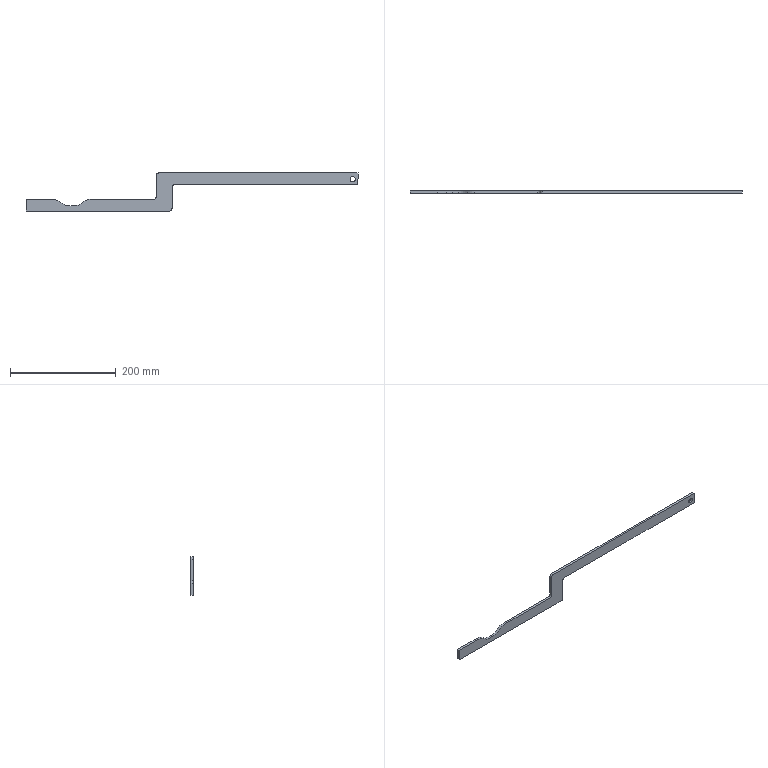Part | SolidWorks | features Extrusion 1 | 1 solid | 24 faces | box 628.5 x 4.5 x 72 mm | volume 66431 mm3 | plane 14 | cylinder 10 | commonest cylinder face diameters 10 x6 40 x4
STEP:
#1=CARTESIAN_POINT('',(618.5,4.5,55.));
#2=VERTEX_POINT('',#1);
#3=CARTESIAN_POINT('',(618.5,4.5,65.));
#4=VERTEX_POINT('',#3);
#5=CARTESIAN_POINT('',(618.5,4.5,60.));
#6=DIRECTION('',(0.,1.,0.));
#7=DIRECTION('',(0.,0.,1.));
#8=AXIS2_PLACEMENT_3D('',#5,#6,#7);
#9=CIRCLE('',#8,5.);
#10=EDGE_CURVE('',#2,#4,#9,.T.);
#11=ORIENTED_EDGE('',*,*,#10,.T.);
#12=CARTESIAN_POINT('',(618.5,0.,65.));
#13=VERTEX_POINT('',#12);
#14=CARTESIAN_POINT('',(618.5,4.5,65.));
#15=DIRECTION('',(0.,-1.,0.));
#16=VECTOR('',#15,1000.);
#17=LINE('',#14,#16);
#18=EDGE_CURVE('',#4,#13,#17,.T.);
#19=ORIENTED_EDGE('',*,*,#18,.T.);
#20=CARTESIAN_POINT('',(618.5,0.,55.));
#21=VERTEX_POINT('',#20);
#22=CARTESIAN_POINT('',(618.5,0.,60.));
#23=DIRECTION('',(0.,1.,0.));
#24=DIRECTION('',(0.,0.,1.));
#25=AXIS2_PLACEMENT_3D('',#22,#23,#24);
#26=CIRCLE('',#25,5.);
#27=EDGE_CURVE('',#21,#13,#26,.T.);
#28=ORIENTED_EDGE('',*,*,#27,.F.);
#29=CARTESIAN_POINT('',(618.5,4.5,55.));
#30=DIRECTION('',(0.,-1.,0.));
#31=VECTOR('',#30,1000.);
#32=LINE('',#29,#31);
#33=EDGE_CURVE('',#2,#21,#32,.T.);
#34=ORIENTED_EDGE('',*,*,#33,.F.);
#35=EDGE_LOOP('',(#11,#19,#28,#34));
#36=FACE_OUTER_BOUND('',#35,.T.);
#37=CARTESIAN_POINT('',(618.5,4.5,60.));
#38=DIRECTION('',(0.,-1.,0.));
#39=DIRECTION('',(0.,0.,-1.));
#40=AXIS2_PLACEMENT_3D('',#37,#38,#39);
#41=CYLINDRICAL_SURFACE('',#40,5.);
#42=ADVANCED_FACE('',(#36),#41,.F.);
#43=CARTESIAN_POINT('',(0.,4.5,0.));
#44=VERTEX_POINT('',#43);
#45=CARTESIAN_POINT('',(0.,4.5,22.));
#46=VERTEX_POINT('',#45);
#47=CARTESIAN_POINT('',(0.,4.5,22.));
#48=DIRECTION('',(0.,0.,1.));
#49=VECTOR('',#48,1000.);
#50=LINE('',#47,#49);
#51=EDGE_CURVE('',#44,#46,#50,.T.);
#52=ORIENTED_EDGE('',*,*,#51,.T.);
#53=CARTESIAN_POINT('',(51.663,4.5,22.));
#54=VERTEX_POINT('',#53);
#55=CARTESIAN_POINT('',(51.663,4.5,22.));
#56=DIRECTION('',(1.,0.,0.));
#57=VECTOR('',#56,1000.);
#58=LINE('',#55,#57);
#59=EDGE_CURVE('',#46,#54,#58,.T.);
#60=ORIENTED_EDGE('',*,*,#59,.T.);
#61=CARTESIAN_POINT('',(63.906,4.5,17.814));
#62=VERTEX_POINT('',#61);
#63=CARTESIAN_POINT('',(51.663,4.5,2.));
#64=DIRECTION('',(0.,1.,0.));
#65=DIRECTION('',(0.,0.,-1.));
#66=AXIS2_PLACEMENT_3D('',#63,#64,#65);
#67=CIRCLE('',#66,20.);
#68=EDGE_CURVE('',#54,#62,#67,.T.);
#69=ORIENTED_EDGE('',*,*,#68,.T.);
#70=CARTESIAN_POINT('',(68.594,4.5,14.186));
#71=VERTEX_POINT('',#70);
#72=CARTESIAN_POINT('',(68.594,4.5,14.186));
#73=DIRECTION('',(0.7907,0.,-0.6122));
#74=VECTOR('',#73,1000.);
#75=LINE('',#72,#74);
#76=EDGE_CURVE('',#62,#71,#75,.T.);
#77=ORIENTED_EDGE('',*,*,#76,.T.);
#78=CARTESIAN_POINT('',(80.837,4.5,10.));
#79=VERTEX_POINT('',#78);
#80=CARTESIAN_POINT('',(80.837,4.5,30.));
#81=DIRECTION('',(0.,-1.,0.));
#82=DIRECTION('',(0.,0.,-1.));
#83=AXIS2_PLACEMENT_3D('',#80,#81,#82);
#84=CIRCLE('',#83,20.);
#85=EDGE_CURVE('',#71,#79,#84,.T.);
#86=ORIENTED_EDGE('',*,*,#85,.T.);
#87=CARTESIAN_POINT('',(92.163,4.5,10.));
#88=VERTEX_POINT('',#87);
#89=CARTESIAN_POINT('',(80.837,4.5,10.));
#90=DIRECTION('',(1.,0.,0.));
#91=VECTOR('',#90,1000.);
#92=LINE('',#89,#91);
#93=EDGE_CURVE('',#79,#88,#92,.T.);
#94=ORIENTED_EDGE('',*,*,#93,.T.);
#95=CARTESIAN_POINT('',(104.406,4.5,14.186));
#96=VERTEX_POINT('',#95);
#97=CARTESIAN_POINT('',(92.163,4.5,30.));
#98=DIRECTION('',(0.,-1.,0.));
#99=DIRECTION('',(0.,0.,-1.));
#100=AXIS2_PLACEMENT_3D('',#97,#98,#99);
#101=CIRCLE('',#100,20.);
#102=EDGE_CURVE('',#88,#96,#101,.T.);
#103=ORIENTED_EDGE('',*,*,#102,.T.);
#104=CARTESIAN_POINT('',(109.094,4.5,17.814));
#105=VERTEX_POINT('',#104);
#106=CARTESIAN_POINT('',(104.406,4.5,14.186));
#107=DIRECTION('',(0.7907,0.,0.6122));
#108=VECTOR('',#107,1000.);
#109=LINE('',#106,#108);
#110=EDGE_CURVE('',#96,#105,#109,.T.);
#111=ORIENTED_EDGE('',*,*,#110,.T.);
#112=CARTESIAN_POINT('',(121.337,4.5,22.));
#113=VERTEX_POINT('',#112);
#114=CARTESIAN_POINT('',(121.337,4.5,2.));
#115=DIRECTION('',(0.,1.,0.));
#116=DIRECTION('',(0.,0.,-1.));
#117=AXIS2_PLACEMENT_3D('',#114,#115,#116);
#118=CIRCLE('',#117,20.);
#119=EDGE_CURVE('',#105,#113,#118,.T.);
#120=ORIENTED_EDGE('',*,*,#119,.T.);
#121=CARTESIAN_POINT('',(241.5,4.5,22.));
#122=VERTEX_POINT('',#121);
#123=CARTESIAN_POINT('',(241.5,4.5,22.));
#124=DIRECTION('',(1.,0.,0.));
#125=VECTOR('',#124,1000.);
#126=LINE('',#123,#125);
#127=EDGE_CURVE('',#113,#122,#126,.T.);
#128=ORIENTED_EDGE('',*,*,#127,.T.);
#129=CARTESIAN_POINT('',(246.5,4.5,27.));
#130=VERTEX_POINT('',#129);
#131=CARTESIAN_POINT('',(241.5,4.5,27.));
#132=DIRECTION('',(0.,-1.,0.));
#133=DIRECTION('',(0.,0.,1.));
#134=AXIS2_PLACEMENT_3D('',#131,#132,#133);
#135=CIRCLE('',#134,5.);
#136=EDGE_CURVE('',#122,#130,#135,.T.);
#137=ORIENTED_EDGE('',*,*,#136,.T.);
#138=CARTESIAN_POINT('',(246.5,4.5,67.));
#139=VERTEX_POINT('',#138);
#140=CARTESIAN_POINT('',(246.5,4.5,67.));
#141=DIRECTION('',(0.,0.,1.));
#142=VECTOR('',#141,1000.);
#143=LINE('',#140,#142);
#144=EDGE_CURVE('',#130,#139,#143,.T.);
#145=ORIENTED_EDGE('',*,*,#144,.T.);
#146=CARTESIAN_POINT('',(251.5,4.5,72.));
#147=VERTEX_POINT('',#146);
#148=CARTESIAN_POINT('',(251.5,4.5,67.));
#149=DIRECTION('',(0.,1.,0.));
#150=DIRECTION('',(0.,0.,-1.));
#151=AXIS2_PLACEMENT_3D('',#148,#149,#150);
#152=CIRCLE('',#151,5.);
#153=EDGE_CURVE('',#139,#147,#152,.T.);
#154=ORIENTED_EDGE('',*,*,#153,.T.);
#155=CARTESIAN_POINT('',(628.5,4.5,72.));
#156=VERTEX_POINT('',#155);
#157=CARTESIAN_POINT('',(628.5,4.5,72.));
#158=DIRECTION('',(1.,0.,0.));
#159=VECTOR('',#158,1000.);
#160=LINE('',#157,#159);
#161=EDGE_CURVE('',#147,#156,#160,.T.);
#162=ORIENTED_EDGE('',*,*,#161,.T.);
#163=CARTESIAN_POINT('',(628.5,4.5,50.));
#164=VERTEX_POINT('',#163);
#165=CARTESIAN_POINT('',(628.5,4.5,50.));
#166=DIRECTION('',(0.,0.,-1.));
#167=VECTOR('',#166,1000.);
#168=LINE('',#165,#167);
#169=EDGE_CURVE('',#156,#164,#168,.T.);
#170=ORIENTED_EDGE('',*,*,#169,.T.);
#171=CARTESIAN_POINT('',(281.5,4.5,50.));
#172=VERTEX_POINT('',#171);
#173=CARTESIAN_POINT('',(281.5,4.5,50.));
#174=DIRECTION('',(-1.,0.,0.));
#175=VECTOR('',#174,1000.);
#176=LINE('',#173,#175);
#177=EDGE_CURVE('',#164,#172,#176,.T.);
#178=ORIENTED_EDGE('',*,*,#177,.T.);
#179=CARTESIAN_POINT('',(276.5,4.5,45.));
#180=VERTEX_POINT('',#179);
#181=CARTESIAN_POINT('',(281.5,4.5,45.));
#182=DIRECTION('',(0.,-1.,0.));
#183=DIRECTION('',(0.,0.,1.));
#184=AXIS2_PLACEMENT_3D('',#181,#182,#183);
#185=CIRCLE('',#184,5.);
#186=EDGE_CURVE('',#172,#180,#185,.T.);
#187=ORIENTED_EDGE('',*,*,#186,.T.);
#188=CARTESIAN_POINT('',(276.5,4.5,5.));
#189=VERTEX_POINT('',#188);
#190=CARTESIAN_POINT('',(276.5,4.5,5.));
#191=DIRECTION('',(0.,0.,-1.));
#192=VECTOR('',#191,1000.);
#193=LINE('',#190,#192);
#194=EDGE_CURVE('',#180,#189,#193,.T.);
#195=ORIENTED_EDGE('',*,*,#194,.T.);
#196=CARTESIAN_POINT('',(271.5,4.5,0.));
#197=VERTEX_POINT('',#196);
#198=CARTESIAN_POINT('',(271.5,4.5,5.));
#199=DIRECTION('',(0.,1.,0.));
#200=DIRECTION('',(0.,0.,-1.));
#201=AXIS2_PLACEMENT_3D('',#198,#199,#200);
#202=CIRCLE('',#201,5.);
#203=EDGE_CURVE('',#189,#197,#202,.T.);
#204=ORIENTED_EDGE('',*,*,#203,.T.);
#205=CARTESIAN_POINT('',(0.,4.5,0.));
#206=DIRECTION('',(-1.,0.,0.));
#207=VECTOR('',#206,1000.);
#208=LINE('',#205,#207);
#209=EDGE_CURVE('',#197,#44,#208,.T.);
#210=ORIENTED_EDGE('',*,*,#209,.T.);
#211=EDGE_LOOP('',(#52,#60,#69,#77,#86,#94,#103,#111,#120,#128,#137,#145,#154,#162,#170,#178,#187,#195,#204,#210));
#212=FACE_OUTER_BOUND('',#211,.T.);
#213=ORIENTED_EDGE('',*,*,#10,.F.);
#214=CARTESIAN_POINT('',(618.5,4.5,60.));
#215=DIRECTION('',(0.,1.,0.));
#216=DIRECTION('',(0.,0.,1.));
#217=AXIS2_PLACEMENT_3D('',#214,#215,#216);
#218=CIRCLE('',#217,5.);
#219=EDGE_CURVE('',#4,#2,#218,.T.);
#220=ORIENTED_EDGE('',*,*,#219,.F.);
#221=EDGE_LOOP('',(#213,#220));
#222=FACE_BOUND('',#221,.T.);
#223=CARTESIAN_POINT('',(271.5,4.5,5.));
#224=DIRECTION('',(0.,-1.,0.));
#225=DIRECTION('',(0.,0.,-1.));
#226=AXIS2_PLACEMENT_3D('',#223,#224,#225);
#227=PLANE('',#226);
#228=ADVANCED_FACE('',(#212,#222),#227,.F.);
#229=CARTESIAN_POINT('',(0.,0.,0.));
#230=VERTEX_POINT('',#229);
#231=CARTESIAN_POINT('',(0.,0.,22.));
#232=VERTEX_POINT('',#231);
#233=CARTESIAN_POINT('',(0.,0.,22.));
#234=DIRECTION('',(0.,0.,1.));
#235=VECTOR('',#234,1000.);
#236=LINE('',#233,#235);
#237=EDGE_CURVE('',#230,#232,#236,.T.);
#238=ORIENTED_EDGE('',*,*,#237,.F.);
#239=CARTESIAN_POINT('',(271.5,0.,0.));
#240=VERTEX_POINT('',#239);
#241=CARTESIAN_POINT('',(0.,0.,0.));
#242=DIRECTION('',(-1.,0.,0.));
#243=VECTOR('',#242,1000.);
#244=LINE('',#241,#243);
#245=EDGE_CURVE('',#240,#230,#244,.T.);
#246=ORIENTED_EDGE('',*,*,#245,.F.);
#247=CARTESIAN_POINT('',(276.5,0.,5.));
#248=VERTEX_POINT('',#247);
#249=CARTESIAN_POINT('',(271.5,0.,5.));
#250=DIRECTION('',(0.,1.,0.));
#251=DIRECTION('',(0.,0.,-1.));
#252=AXIS2_PLACEMENT_3D('',#249,#250,#251);
#253=CIRCLE('',#252,5.);
#254=EDGE_CURVE('',#248,#240,#253,.T.);
#255=ORIENTED_EDGE('',*,*,#254,.F.);
#256=CARTESIAN_POINT('',(276.5,0.,45.));
#257=VERTEX_POINT('',#256);
#258=CARTESIAN_POINT('',(276.5,0.,5.));
#259=DIRECTION('',(0.,0.,-1.));
#260=VECTOR('',#259,1000.);
#261=LINE('',#258,#260);
#262=EDGE_CURVE('',#257,#248,#261,.T.);
#263=ORIENTED_EDGE('',*,*,#262,.F.);
#264=CARTESIAN_POINT('',(281.5,0.,50.));
#265=VERTEX_POINT('',#264);
#266=CARTESIAN_POINT('',(281.5,0.,45.));
#267=DIRECTION('',(0.,-1.,0.));
#268=DIRECTION('',(0.,0.,1.));
#269=AXIS2_PLACEMENT_3D('',#266,#267,#268);
#270=CIRCLE('',#269,5.);
#271=EDGE_CURVE('',#265,#257,#270,.T.);
#272=ORIENTED_EDGE('',*,*,#271,.F.);
#273=CARTESIAN_POINT('',(628.5,0.,50.));
#274=VERTEX_POINT('',#273);
#275=CARTESIAN_POINT('',(281.5,0.,50.));
#276=DIRECTION('',(-1.,0.,0.));
#277=VECTOR('',#276,1000.);
#278=LINE('',#275,#277);
#279=EDGE_CURVE('',#274,#265,#278,.T.);
#280=ORIENTED_EDGE('',*,*,#279,.F.);
#281=CARTESIAN_POINT('',(628.5,0.,72.));
#282=VERTEX_POINT('',#281);
#283=CARTESIAN_POINT('',(628.5,0.,50.));
#284=DIRECTION('',(0.,0.,-1.));
#285=VECTOR('',#284,1000.);
#286=LINE('',#283,#285);
#287=EDGE_CURVE('',#282,#274,#286,.T.);
#288=ORIENTED_EDGE('',*,*,#287,.F.);
#289=CARTESIAN_POINT('',(251.5,0.,72.));
#290=VERTEX_POINT('',#289);
#291=CARTESIAN_POINT('',(628.5,0.,72.));
#292=DIRECTION('',(1.,0.,0.));
#293=VECTOR('',#292,1000.);
#294=LINE('',#291,#293);
#295=EDGE_CURVE('',#290,#282,#294,.T.);
#296=ORIENTED_EDGE('',*,*,#295,.F.);
#297=CARTESIAN_POINT('',(246.5,0.,67.));
#298=VERTEX_POINT('',#297);
#299=CARTESIAN_POINT('',(251.5,0.,67.));
#300=DIRECTION('',(0.,1.,0.));
#301=DIRECTION('',(0.,0.,-1.));
#302=AXIS2_PLACEMENT_3D('',#299,#300,#301);
#303=CIRCLE('',#302,5.);
#304=EDGE_CURVE('',#298,#290,#303,.T.);
#305=ORIENTED_EDGE('',*,*,#304,.F.);
#306=CARTESIAN_POINT('',(246.5,0.,27.));
#307=VERTEX_POINT('',#306);
#308=CARTESIAN_POINT('',(246.5,0.,67.));
#309=DIRECTION('',(0.,0.,1.));
#310=VECTOR('',#309,1000.);
#311=LINE('',#308,#310);
#312=EDGE_CURVE('',#307,#298,#311,.T.);
#313=ORIENTED_EDGE('',*,*,#312,.F.);
#314=CARTESIAN_POINT('',(241.5,0.,22.));
#315=VERTEX_POINT('',#314);
#316=CARTESIAN_POINT('',(241.5,0.,27.));
#317=DIRECTION('',(0.,-1.,0.));
#318=DIRECTION('',(0.,0.,1.));
#319=AXIS2_PLACEMENT_3D('',#316,#317,#318);
#320=CIRCLE('',#319,5.);
#321=EDGE_CURVE('',#315,#307,#320,.T.);
#322=ORIENTED_EDGE('',*,*,#321,.F.);
#323=CARTESIAN_POINT('',(121.337,0.,22.));
#324=VERTEX_POINT('',#323);
#325=CARTESIAN_POINT('',(241.5,0.,22.));
#326=DIRECTION('',(1.,0.,0.));
#327=VECTOR('',#326,1000.);
#328=LINE('',#325,#327);
#329=EDGE_CURVE('',#324,#315,#328,.T.);
#330=ORIENTED_EDGE('',*,*,#329,.F.);
#331=CARTESIAN_POINT('',(109.094,0.,17.814));
#332=VERTEX_POINT('',#331);
#333=CARTESIAN_POINT('',(121.337,0.,2.));
#334=DIRECTION('',(0.,1.,0.));
#335=DIRECTION('',(0.,0.,-1.));
#336=AXIS2_PLACEMENT_3D('',#333,#334,#335);
#337=CIRCLE('',#336,20.);
#338=EDGE_CURVE('',#332,#324,#337,.T.);
#339=ORIENTED_EDGE('',*,*,#338,.F.);
#340=CARTESIAN_POINT('',(104.406,0.,14.186));
#341=VERTEX_POINT('',#340);
#342=CARTESIAN_POINT('',(104.406,0.,14.186));
#343=DIRECTION('',(0.7907,0.,0.6122));
#344=VECTOR('',#343,1000.);
#345=LINE('',#342,#344);
#346=EDGE_CURVE('',#341,#332,#345,.T.);
#347=ORIENTED_EDGE('',*,*,#346,.F.);
#348=CARTESIAN_POINT('',(92.163,0.,10.));
#349=VERTEX_POINT('',#348);
#350=CARTESIAN_POINT('',(92.163,0.,30.));
#351=DIRECTION('',(0.,-1.,0.));
#352=DIRECTION('',(0.,0.,-1.));
#353=AXIS2_PLACEMENT_3D('',#350,#351,#352);
#354=CIRCLE('',#353,20.);
#355=EDGE_CURVE('',#349,#341,#354,.T.);
#356=ORIENTED_EDGE('',*,*,#355,.F.);
#357=CARTESIAN_POINT('',(80.837,0.,10.));
#358=VERTEX_POINT('',#357);
#359=CARTESIAN_POINT('',(80.837,0.,10.));
#360=DIRECTION('',(1.,0.,0.));
#361=VECTOR('',#360,1000.);
#362=LINE('',#359,#361);
#363=EDGE_CURVE('',#358,#349,#362,.T.);
#364=ORIENTED_EDGE('',*,*,#363,.F.);
#365=CARTESIAN_POINT('',(68.594,0.,14.186));
#366=VERTEX_POINT('',#365);
#367=CARTESIAN_POINT('',(80.837,0.,30.));
#368=DIRECTION('',(0.,-1.,0.));
#369=DIRECTION('',(0.,0.,-1.));
#370=AXIS2_PLACEMENT_3D('',#367,#368,#369);
#371=CIRCLE('',#370,20.);
#372=EDGE_CURVE('',#366,#358,#371,.T.);
#373=ORIENTED_EDGE('',*,*,#372,.F.);
#374=CARTESIAN_POINT('',(63.906,0.,17.814));
#375=VERTEX_POINT('',#374);
#376=CARTESIAN_POINT('',(68.594,0.,14.186));
#377=DIRECTION('',(0.7907,0.,-0.6122));
#378=VECTOR('',#377,1000.);
#379=LINE('',#376,#378);
#380=EDGE_CURVE('',#375,#366,#379,.T.);
#381=ORIENTED_EDGE('',*,*,#380,.F.);
#382=CARTESIAN_POINT('',(51.663,0.,22.));
#383=VERTEX_POINT('',#382);
#384=CARTESIAN_POINT('',(51.663,0.,2.));
#385=DIRECTION('',(0.,1.,0.));
#386=DIRECTION('',(0.,0.,-1.));
#387=AXIS2_PLACEMENT_3D('',#384,#385,#386);
#388=CIRCLE('',#387,20.);
#389=EDGE_CURVE('',#383,#375,#388,.T.);
#390=ORIENTED_EDGE('',*,*,#389,.F.);
#391=CARTESIAN_POINT('',(51.663,0.,22.));
#392=DIRECTION('',(1.,0.,0.));
#393=VECTOR('',#392,1000.);
#394=LINE('',#391,#393);
#395=EDGE_CURVE('',#232,#383,#394,.T.);
#396=ORIENTED_EDGE('',*,*,#395,.F.);
#397=EDGE_LOOP('',(#238,#246,#255,#263,#272,#280,#288,#296,#305,#313,#322,#330,#339,#347,#356,#364,#373,#381,#390,#396));
#398=FACE_OUTER_BOUND('',#397,.T.);
#399=ORIENTED_EDGE('',*,*,#27,.T.);
#400=CARTESIAN_POINT('',(618.5,0.,60.));
#401=DIRECTION('',(0.,1.,0.));
#402=DIRECTION('',(0.,0.,1.));
#403=AXIS2_PLACEMENT_3D('',#400,#401,#402);
#404=CIRCLE('',#403,5.);
#405=EDGE_CURVE('',#13,#21,#404,.T.);
#406=ORIENTED_EDGE('',*,*,#405,.T.);
#407=EDGE_LOOP('',(#399,#406));
#408=FACE_BOUND('',#407,.T.);
#409=CARTESIAN_POINT('',(271.5,0.,5.));
#410=DIRECTION('',(0.,-1.,0.));
#411=DIRECTION('',(0.,0.,-1.));
#412=AXIS2_PLACEMENT_3D('',#409,#410,#411);
#413=PLANE('',#412);
#414=ADVANCED_FACE('',(#398,#408),#413,.T.);
#415=ORIENTED_EDGE('',*,*,#237,.T.);
#416=CARTESIAN_POINT('',(0.,4.5,22.));
#417=DIRECTION('',(0.,-1.,0.));
#418=VECTOR('',#417,1000.);
#419=LINE('',#416,#418);
#420=EDGE_CURVE('',#46,#232,#419,.T.);
#421=ORIENTED_EDGE('',*,*,#420,.F.);
#422=ORIENTED_EDGE('',*,*,#51,.F.);
#423=CARTESIAN_POINT('',(0.,4.5,0.));
#424=DIRECTION('',(0.,-1.,0.));
#425=VECTOR('',#424,1000.);
#426=LINE('',#423,#425);
#427=EDGE_CURVE('',#44,#230,#426,.T.);
#428=ORIENTED_EDGE('',*,*,#427,.T.);
#429=EDGE_LOOP('',(#415,#421,#422,#428));
#430=FACE_OUTER_BOUND('',#429,.T.);
#431=CARTESIAN_POINT('',(0.,4.5,22.));
#432=DIRECTION('',(1.,0.,0.));
#433=DIRECTION('',(0.,0.,-1.));
#434=AXIS2_PLACEMENT_3D('',#431,#432,#433);
#435=PLANE('',#434);
#436=ADVANCED_FACE('',(#430),#435,.F.);
#437=ORIENTED_EDGE('',*,*,#395,.T.);
#438=CARTESIAN_POINT('',(51.663,4.5,22.));
#439=DIRECTION('',(0.,-1.,0.));
#440=VECTOR('',#439,1000.);
#441=LINE('',#438,#440);
#442=EDGE_CURVE('',#54,#383,#441,.T.);
#443=ORIENTED_EDGE('',*,*,#442,.F.);
#444=ORIENTED_EDGE('',*,*,#59,.F.);
#445=ORIENTED_EDGE('',*,*,#420,.T.);
#446=EDGE_LOOP('',(#437,#443,#444,#445));
#447=FACE_OUTER_BOUND('',#446,.T.);
#448=CARTESIAN_POINT('',(51.663,4.5,22.));
#449=DIRECTION('',(0.,0.,-1.));
#450=DIRECTION('',(-1.,0.,0.));
#451=AXIS2_PLACEMENT_3D('',#448,#449,#450);
#452=PLANE('',#451);
#453=ADVANCED_FACE('',(#447),#452,.F.);
#454=ORIENTED_EDGE('',*,*,#389,.T.);
#455=CARTESIAN_POINT('',(63.906,4.5,17.814));
#456=DIRECTION('',(0.,-1.,0.));
#457=VECTOR('',#456,1000.);
#458=LINE('',#455,#457);
#459=EDGE_CURVE('',#62,#375,#458,.T.);
#460=ORIENTED_EDGE('',*,*,#459,.F.);
#461=ORIENTED_EDGE('',*,*,#68,.F.);
#462=ORIENTED_EDGE('',*,*,#442,.T.);
#463=EDGE_LOOP('',(#454,#460,#461,#462));
#464=FACE_OUTER_BOUND('',#463,.T.);
#465=CARTESIAN_POINT('',(51.663,4.5,2.));
#466=DIRECTION('',(0.,-1.,0.));
#467=DIRECTION('',(0.,0.,-1.));
#468=AXIS2_PLACEMENT_3D('',#465,#466,#467);
#469=CYLINDRICAL_SURFACE('',#468,20.);
#470=ADVANCED_FACE('',(#464),#469,.T.);
#471=ORIENTED_EDGE('',*,*,#380,.T.);
#472=CARTESIAN_POINT('',(68.594,4.5,14.186));
#473=DIRECTION('',(0.,-1.,0.));
#474=VECTOR('',#473,1000.);
#475=LINE('',#472,#474);
#476=EDGE_CURVE('',#71,#366,#475,.T.);
#477=ORIENTED_EDGE('',*,*,#476,.F.);
#478=ORIENTED_EDGE('',*,*,#76,.F.);
#479=ORIENTED_EDGE('',*,*,#459,.T.);
#480=EDGE_LOOP('',(#471,#477,#478,#479));
#481=FACE_OUTER_BOUND('',#480,.T.);
#482=CARTESIAN_POINT('',(68.594,4.5,14.186));
#483=DIRECTION('',(-0.6122,0.,-0.7907));
#484=DIRECTION('',(-0.7907,0.,0.6122));
#485=AXIS2_PLACEMENT_3D('',#482,#483,#484);
#486=PLANE('',#485);
#487=ADVANCED_FACE('',(#481),#486,.F.);
#488=ORIENTED_EDGE('',*,*,#372,.T.);
#489=CARTESIAN_POINT('',(80.837,4.5,10.));
#490=DIRECTION('',(0.,-1.,0.));
#491=VECTOR('',#490,1000.);
#492=LINE('',#489,#491);
#493=EDGE_CURVE('',#79,#358,#492,.T.);
#494=ORIENTED_EDGE('',*,*,#493,.F.);
#495=ORIENTED_EDGE('',*,*,#85,.F.);
#496=ORIENTED_EDGE('',*,*,#476,.T.);
#497=EDGE_LOOP('',(#488,#494,#495,#496));
#498=FACE_OUTER_BOUND('',#497,.T.);
#499=CARTESIAN_POINT('',(80.837,4.5,30.));
#500=DIRECTION('',(0.,-1.,0.));
#501=DIRECTION('',(0.,0.,-1.));
#502=AXIS2_PLACEMENT_3D('',#499,#500,#501);
#503=CYLINDRICAL_SURFACE('',#502,20.);
#504=ADVANCED_FACE('',(#498),#503,.F.);
#505=ORIENTED_EDGE('',*,*,#363,.T.);
#506=CARTESIAN_POINT('',(92.163,4.5,10.));
#507=DIRECTION('',(0.,-1.,0.));
#508=VECTOR('',#507,1000.);
#509=LINE('',#506,#508);
#510=EDGE_CURVE('',#88,#349,#509,.T.);
#511=ORIENTED_EDGE('',*,*,#510,.F.);
#512=ORIENTED_EDGE('',*,*,#93,.F.);
#513=ORIENTED_EDGE('',*,*,#493,.T.);
#514=EDGE_LOOP('',(#505,#511,#512,#513));
#515=FACE_OUTER_BOUND('',#514,.T.);
#516=CARTESIAN_POINT('',(80.837,4.5,10.));
#517=DIRECTION('',(0.,0.,-1.));
#518=DIRECTION('',(-1.,0.,0.));
#519=AXIS2_PLACEMENT_3D('',#516,#517,#518);
#520=PLANE('',#519);
#521=ADVANCED_FACE('',(#515),#520,.F.);
#522=ORIENTED_EDGE('',*,*,#355,.T.);
#523=CARTESIAN_POINT('',(104.406,4.5,14.186));
#524=DIRECTION('',(0.,-1.,0.));
#525=VECTOR('',#524,1000.);
#526=LINE('',#523,#525);
#527=EDGE_CURVE('',#96,#341,#526,.T.);
#528=ORIENTED_EDGE('',*,*,#527,.F.);
#529=ORIENTED_EDGE('',*,*,#102,.F.);
#530=ORIENTED_EDGE('',*,*,#510,.T.);
#531=EDGE_LOOP('',(#522,#528,#529,#530));
#532=FACE_OUTER_BOUND('',#531,.T.);
#533=CARTESIAN_POINT('',(92.163,4.5,30.));
#534=DIRECTION('',(0.,-1.,0.));
#535=DIRECTION('',(0.,0.,-1.));
#536=AXIS2_PLACEMENT_3D('',#533,#534,#535);
#537=CYLINDRICAL_SURFACE('',#536,20.);
#538=ADVANCED_FACE('',(#532),#537,.F.);
#539=ORIENTED_EDGE('',*,*,#346,.T.);
#540=CARTESIAN_POINT('',(109.094,4.5,17.814));
#541=DIRECTION('',(0.,-1.,0.));
#542=VECTOR('',#541,1000.);
#543=LINE('',#540,#542);
#544=EDGE_CURVE('',#105,#332,#543,.T.);
#545=ORIENTED_EDGE('',*,*,#544,.F.);
#546=ORIENTED_EDGE('',*,*,#110,.F.);
#547=ORIENTED_EDGE('',*,*,#527,.T.);
#548=EDGE_LOOP('',(#539,#545,#546,#547));
#549=FACE_OUTER_BOUND('',#548,.T.);
#550=CARTESIAN_POINT('',(104.406,4.5,14.186));
#551=DIRECTION('',(0.6122,0.,-0.7907));
#552=DIRECTION('',(-0.7907,0.,-0.6122));
#553=AXIS2_PLACEMENT_3D('',#550,#551,#552);
#554=PLANE('',#553);
#555=ADVANCED_FACE('',(#549),#554,.F.);
#556=ORIENTED_EDGE('',*,*,#338,.T.);
#557=CARTESIAN_POINT('',(121.337,4.5,22.));
#558=DIRECTION('',(0.,-1.,0.));
#559=VECTOR('',#558,1000.);
#560=LINE('',#557,#559);
#561=EDGE_CURVE('',#113,#324,#560,.T.);
#562=ORIENTED_EDGE('',*,*,#561,.F.);
#563=ORIENTED_EDGE('',*,*,#119,.F.);
#564=ORIENTED_EDGE('',*,*,#544,.T.);
#565=EDGE_LOOP('',(#556,#562,#563,#564));
#566=FACE_OUTER_BOUND('',#565,.T.);
#567=CARTESIAN_POINT('',(121.337,4.5,2.));
#568=DIRECTION('',(0.,-1.,0.));
#569=DIRECTION('',(0.,0.,-1.));
#570=AXIS2_PLACEMENT_3D('',#567,#568,#569);
#571=CYLINDRICAL_SURFACE('',#570,20.);
#572=ADVANCED_FACE('',(#566),#571,.T.);
#573=ORIENTED_EDGE('',*,*,#329,.T.);
#574=CARTESIAN_POINT('',(241.5,4.5,22.));
#575=DIRECTION('',(0.,-1.,0.));
#576=VECTOR('',#575,1000.);
#577=LINE('',#574,#576);
#578=EDGE_CURVE('',#122,#315,#577,.T.);
#579=ORIENTED_EDGE('',*,*,#578,.F.);
#580=ORIENTED_EDGE('',*,*,#127,.F.);
#581=ORIENTED_EDGE('',*,*,#561,.T.);
#582=EDGE_LOOP('',(#573,#579,#580,#581));
#583=FACE_OUTER_BOUND('',#582,.T.);
#584=CARTESIAN_POINT('',(241.5,4.5,22.));
#585=DIRECTION('',(0.,0.,-1.));
#586=DIRECTION('',(-1.,0.,0.));
#587=AXIS2_PLACEMENT_3D('',#584,#585,#586);
#588=PLANE('',#587);
#589=ADVANCED_FACE('',(#583),#588,.F.);
#590=ORIENTED_EDGE('',*,*,#321,.T.);
#591=CARTESIAN_POINT('',(246.5,4.5,27.));
#592=DIRECTION('',(0.,-1.,0.));
#593=VECTOR('',#592,1000.);
#594=LINE('',#591,#593);
#595=EDGE_CURVE('',#130,#307,#594,.T.);
#596=ORIENTED_EDGE('',*,*,#595,.F.);
#597=ORIENTED_EDGE('',*,*,#136,.F.);
#598=ORIENTED_EDGE('',*,*,#578,.T.);
#599=EDGE_LOOP('',(#590,#596,#597,#598));
#600=FACE_OUTER_BOUND('',#599,.T.);
#601=CARTESIAN_POINT('',(241.5,4.5,27.));
#602=DIRECTION('',(0.,-1.,0.));
#603=DIRECTION('',(0.,0.,-1.));
#604=AXIS2_PLACEMENT_3D('',#601,#602,#603);
#605=CYLINDRICAL_SURFACE('',#604,5.);
#606=ADVANCED_FACE('',(#600),#605,.F.);
#607=ORIENTED_EDGE('',*,*,#312,.T.);
#608=CARTESIAN_POINT('',(246.5,4.5,67.));
#609=DIRECTION('',(0.,-1.,0.));
#610=VECTOR('',#609,1000.);
#611=LINE('',#608,#610);
#612=EDGE_CURVE('',#139,#298,#611,.T.);
#613=ORIENTED_EDGE('',*,*,#612,.F.);
#614=ORIENTED_EDGE('',*,*,#144,.F.);
#615=ORIENTED_EDGE('',*,*,#595,.T.);
#616=EDGE_LOOP('',(#607,#613,#614,#615));
#617=FACE_OUTER_BOUND('',#616,.T.);
#618=CARTESIAN_POINT('',(246.5,4.5,67.));
#619=DIRECTION('',(1.,0.,0.));
#620=DIRECTION('',(0.,0.,-1.));
#621=AXIS2_PLACEMENT_3D('',#618,#619,#620);
#622=PLANE('',#621);
#623=ADVANCED_FACE('',(#617),#622,.F.);
#624=ORIENTED_EDGE('',*,*,#304,.T.);
#625=CARTESIAN_POINT('',(251.5,4.5,72.));
#626=DIRECTION('',(0.,-1.,0.));
#627=VECTOR('',#626,1000.);
#628=LINE('',#625,#627);
#629=EDGE_CURVE('',#147,#290,#628,.T.);
#630=ORIENTED_EDGE('',*,*,#629,.F.);
#631=ORIENTED_EDGE('',*,*,#153,.F.);
#632=ORIENTED_EDGE('',*,*,#612,.T.);
#633=EDGE_LOOP('',(#624,#630,#631,#632));
#634=FACE_OUTER_BOUND('',#633,.T.);
#635=CARTESIAN_POINT('',(251.5,4.5,67.));
#636=DIRECTION('',(0.,-1.,0.));
#637=DIRECTION('',(0.,0.,-1.));
#638=AXIS2_PLACEMENT_3D('',#635,#636,#637);
#639=CYLINDRICAL_SURFACE('',#638,5.);
#640=ADVANCED_FACE('',(#634),#639,.T.);
#641=ORIENTED_EDGE('',*,*,#295,.T.);
#642=CARTESIAN_POINT('',(628.5,4.5,72.));
#643=DIRECTION('',(0.,-1.,0.));
#644=VECTOR('',#643,1000.);
#645=LINE('',#642,#644);
#646=EDGE_CURVE('',#156,#282,#645,.T.);
#647=ORIENTED_EDGE('',*,*,#646,.F.);
#648=ORIENTED_EDGE('',*,*,#161,.F.);
#649=ORIENTED_EDGE('',*,*,#629,.T.);
#650=EDGE_LOOP('',(#641,#647,#648,#649));
#651=FACE_OUTER_BOUND('',#650,.T.);
#652=CARTESIAN_POINT('',(628.5,4.5,72.));
#653=DIRECTION('',(0.,0.,-1.));
#654=DIRECTION('',(-1.,0.,0.));
#655=AXIS2_PLACEMENT_3D('',#652,#653,#654);
#656=PLANE('',#655);
#657=ADVANCED_FACE('',(#651),#656,.F.);
#658=ORIENTED_EDGE('',*,*,#287,.T.);
#659=CARTESIAN_POINT('',(628.5,4.5,50.));
#660=DIRECTION('',(0.,-1.,0.));
#661=VECTOR('',#660,1000.);
#662=LINE('',#659,#661);
#663=EDGE_CURVE('',#164,#274,#662,.T.);
#664=ORIENTED_EDGE('',*,*,#663,.F.);
#665=ORIENTED_EDGE('',*,*,#169,.F.);
#666=ORIENTED_EDGE('',*,*,#646,.T.);
#667=EDGE_LOOP('',(#658,#664,#665,#666));
#668=FACE_OUTER_BOUND('',#667,.T.);
#669=CARTESIAN_POINT('',(628.5,4.5,50.));
#670=DIRECTION('',(-1.,0.,0.));
#671=DIRECTION('',(0.,0.,1.));
#672=AXIS2_PLACEMENT_3D('',#669,#670,#671);
#673=PLANE('',#672);
#674=ADVANCED_FACE('',(#668),#673,.F.);
#675=ORIENTED_EDGE('',*,*,#279,.T.);
#676=CARTESIAN_POINT('',(281.5,4.5,50.));
#677=DIRECTION('',(0.,-1.,0.));
#678=VECTOR('',#677,1000.);
#679=LINE('',#676,#678);
#680=EDGE_CURVE('',#172,#265,#679,.T.);
#681=ORIENTED_EDGE('',*,*,#680,.F.);
#682=ORIENTED_EDGE('',*,*,#177,.F.);
#683=ORIENTED_EDGE('',*,*,#663,.T.);
#684=EDGE_LOOP('',(#675,#681,#682,#683));
#685=FACE_OUTER_BOUND('',#684,.T.);
#686=CARTESIAN_POINT('',(281.5,4.5,50.));
#687=DIRECTION('',(0.,0.,1.));
#688=DIRECTION('',(1.,0.,0.));
#689=AXIS2_PLACEMENT_3D('',#686,#687,#688);
#690=PLANE('',#689);
#691=ADVANCED_FACE('',(#685),#690,.F.);
#692=ORIENTED_EDGE('',*,*,#271,.T.);
#693=CARTESIAN_POINT('',(276.5,4.5,45.));
#694=DIRECTION('',(0.,-1.,0.));
#695=VECTOR('',#694,1000.);
#696=LINE('',#693,#695);
#697=EDGE_CURVE('',#180,#257,#696,.T.);
#698=ORIENTED_EDGE('',*,*,#697,.F.);
#699=ORIENTED_EDGE('',*,*,#186,.F.);
#700=ORIENTED_EDGE('',*,*,#680,.T.);
#701=EDGE_LOOP('',(#692,#698,#699,#700));
#702=FACE_OUTER_BOUND('',#701,.T.);
#703=CARTESIAN_POINT('',(281.5,4.5,45.));
#704=DIRECTION('',(0.,-1.,0.));
#705=DIRECTION('',(0.,0.,-1.));
#706=AXIS2_PLACEMENT_3D('',#703,#704,#705);
#707=CYLINDRICAL_SURFACE('',#706,5.);
#708=ADVANCED_FACE('',(#702),#707,.F.);
#709=ORIENTED_EDGE('',*,*,#262,.T.);
#710=CARTESIAN_POINT('',(276.5,4.5,5.));
#711=DIRECTION('',(0.,-1.,0.));
#712=VECTOR('',#711,1000.);
#713=LINE('',#710,#712);
#714=EDGE_CURVE('',#189,#248,#713,.T.);
#715=ORIENTED_EDGE('',*,*,#714,.F.);
#716=ORIENTED_EDGE('',*,*,#194,.F.);
#717=ORIENTED_EDGE('',*,*,#697,.T.);
#718=EDGE_LOOP('',(#709,#715,#716,#717));
#719=FACE_OUTER_BOUND('',#718,.T.);
#720=CARTESIAN_POINT('',(276.5,4.5,5.));
#721=DIRECTION('',(-1.,0.,0.));
#722=DIRECTION('',(0.,0.,1.));
#723=AXIS2_PLACEMENT_3D('',#720,#721,#722);
#724=PLANE('',#723);
#725=ADVANCED_FACE('',(#719),#724,.F.);
#726=ORIENTED_EDGE('',*,*,#254,.T.);
#727=CARTESIAN_POINT('',(271.5,4.5,0.));
#728=DIRECTION('',(0.,-1.,0.));
#729=VECTOR('',#728,1000.);
#730=LINE('',#727,#729);
#731=EDGE_CURVE('',#197,#240,#730,.T.);
#732=ORIENTED_EDGE('',*,*,#731,.F.);
#733=ORIENTED_EDGE('',*,*,#203,.F.);
#734=ORIENTED_EDGE('',*,*,#714,.T.);
#735=EDGE_LOOP('',(#726,#732,#733,#734));
#736=FACE_OUTER_BOUND('',#735,.T.);
#737=CARTESIAN_POINT('',(271.5,4.5,5.));
#738=DIRECTION('',(0.,-1.,0.));
#739=DIRECTION('',(0.,0.,-1.));
#740=AXIS2_PLACEMENT_3D('',#737,#738,#739);
#741=CYLINDRICAL_SURFACE('',#740,5.);
#742=ADVANCED_FACE('',(#736),#741,.T.);
#743=ORIENTED_EDGE('',*,*,#245,.T.);
#744=ORIENTED_EDGE('',*,*,#427,.F.);
#745=ORIENTED_EDGE('',*,*,#209,.F.);
#746=ORIENTED_EDGE('',*,*,#731,.T.);
#747=EDGE_LOOP('',(#743,#744,#745,#746));
#748=FACE_OUTER_BOUND('',#747,.T.);
#749=CARTESIAN_POINT('',(0.,4.5,0.));
#750=DIRECTION('',(0.,0.,1.));
#751=DIRECTION('',(1.,0.,0.));
#752=AXIS2_PLACEMENT_3D('',#749,#750,#751);
#753=PLANE('',#752);
#754=ADVANCED_FACE('',(#748),#753,.F.);
#755=ORIENTED_EDGE('',*,*,#18,.F.);
#756=ORIENTED_EDGE('',*,*,#219,.T.);
#757=ORIENTED_EDGE('',*,*,#33,.T.);
#758=ORIENTED_EDGE('',*,*,#405,.F.);
#759=EDGE_LOOP('',(#755,#756,#757,#758));
#760=FACE_OUTER_BOUND('',#759,.T.);
#761=CARTESIAN_POINT('',(618.5,4.5,60.));
#762=DIRECTION('',(0.,-1.,0.));
#763=DIRECTION('',(0.,0.,-1.));
#764=AXIS2_PLACEMENT_3D('',#761,#762,#763);
#765=CYLINDRICAL_SURFACE('',#764,5.);
#766=ADVANCED_FACE('',(#760),#765,.F.);
#767=CLOSED_SHELL('',(#42,#228,#414,#436,#453,#470,#487,#504,#521,#538,#555,#572,#589,#606,#623,#640,#657,#674,#691,#708,#725,#742,#754,#766));
#768=MANIFOLD_SOLID_BREP('',#767);
#769=CARTESIAN_POINT('',(0.,0.,0.));
#770=DIRECTION('',(0.,0.,1.));
#771=DIRECTION('',(1.,0.,0.));
#772=AXIS2_PLACEMENT_3D('',#769,#770,#771);
#773=(LENGTH_UNIT()NAMED_UNIT(*)SI_UNIT(.MILLI.,.METRE.));
#774=UNCERTAINTY_MEASURE_WITH_UNIT(LENGTH_MEASURE(0.00001),#773,'','');
#775=(NAMED_UNIT(*)PLANE_ANGLE_UNIT()SI_UNIT($,.RADIAN.));
#776=(NAMED_UNIT(*)SI_UNIT($,.STERADIAN.)SOLID_ANGLE_UNIT());
#777=(GEOMETRIC_REPRESENTATION_CONTEXT(3)GLOBAL_UNCERTAINTY_ASSIGNED_CONTEXT((#774))GLOBAL_UNIT_ASSIGNED_CONTEXT((#773,#775,#776))REPRESENTATION_CONTEXT('',''));
#778=ADVANCED_BREP_SHAPE_REPRESENTATION('',(#768,#772),#777);